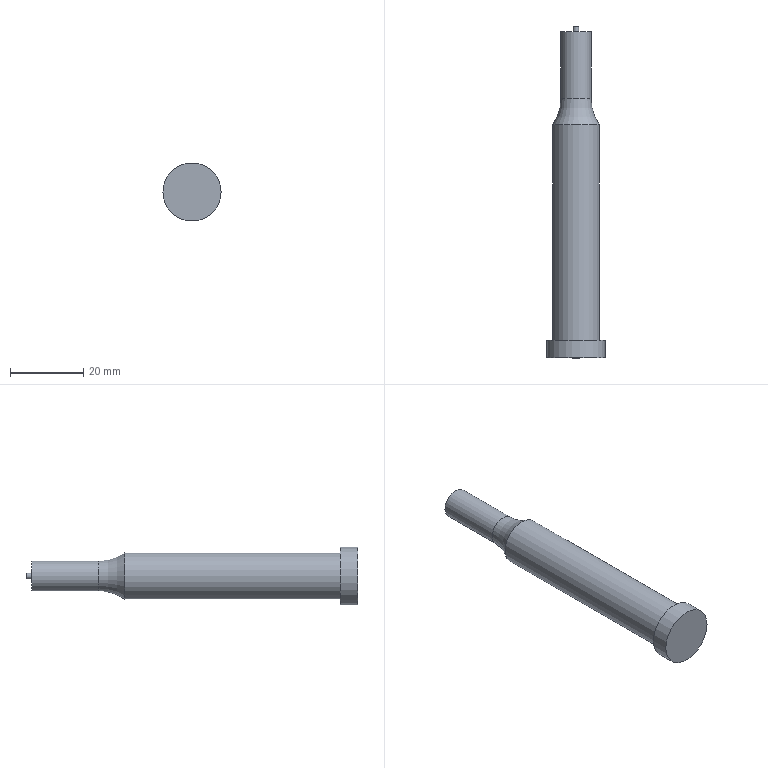Part | STEP file | 1_id1150_x_t | 1 solid | 9 faces | box 15.875 x 90.424 x 15.875 mm | volume 9884 mm3 | plane 4 | cylinder 4 | torus 1 | commonest cylinder face diameters 1.473 x1 8.199 x1 12.7 x1 15.875 x1
STEP:
#1=CARTESIAN_POINT('',(0.,0.,0.));
#2=DIRECTION('',(0.,0.,1.));
#3=DIRECTION('',(1.,0.,0.));
#4=AXIS2_PLACEMENT_3D('',#1,#2,#3);
#5=CARTESIAN_POINT('',(773.362,73.473,-70.67));
#6=VERTEX_POINT('',#5);
#7=CARTESIAN_POINT('',(757.487,73.473,-70.67));
#8=VERTEX_POINT('',#7);
#9=CARTESIAN_POINT('',(765.425,73.473,-70.67));
#10=DIRECTION('',(0.,-1.,0.));
#11=DIRECTION('',(1.,0.,0.));
#12=AXIS2_PLACEMENT_3D('',#9,#10,#11);
#13=CIRCLE('',#12,7.938);
#14=CARTESIAN_POINT('',(762.856,73.473,-70.67));
#15=DIRECTION('',(0.,-1.,0.));
#16=DIRECTION('',(1.,0.,0.));
#17=AXIS2_PLACEMENT_3D('',#14,#15,#16);
#18=PLANE('',#17);
#19=CARTESIAN_POINT('',(2.569,0.));
#20=DIRECTION('',(1.,0.));
#21=AXIS2_PLACEMENT_2D('',#19,#20);
#22=CIRCLE('',#21,7.938);
#23=(GEOMETRIC_REPRESENTATION_CONTEXT(2)PARAMETRIC_REPRESENTATION_CONTEXT()REPRESENTATION_CONTEXT('',''));
#24=DEFINITIONAL_REPRESENTATION('',(#22),#23);
#25=PCURVE('',#18,#24);
#26=CARTESIAN_POINT('',(765.425,75.861,-70.67));
#27=DIRECTION('',(0.,-1.,0.));
#28=DIRECTION('',(-1.,0.,0.));
#29=AXIS2_PLACEMENT_3D('',#26,#27,#28);
#30=CYLINDRICAL_SURFACE('',#29,7.938);
#31=CARTESIAN_POINT('',(3.142,2.388));
#32=DIRECTION('',(1.,0.));
#33=VECTOR('',#32,1.);
#34=LINE('',#31,#33);
#35=(GEOMETRIC_REPRESENTATION_CONTEXT(2)PARAMETRIC_REPRESENTATION_CONTEXT()REPRESENTATION_CONTEXT('',''));
#36=DEFINITIONAL_REPRESENTATION('',(#34),#35);
#37=PCURVE('',#30,#36);
#38=SURFACE_CURVE('',#13,(#25,#37),.PCURVE_S1.);
#39=EDGE_CURVE('',#6,#8,#38,.T.);
#40=ORIENTED_EDGE('',*,*,#39,.T.);
#41=CARTESIAN_POINT('',(765.425,73.473,-70.67));
#42=DIRECTION('',(0.,-1.,0.));
#43=DIRECTION('',(1.,0.,0.));
#44=AXIS2_PLACEMENT_3D('',#41,#42,#43);
#45=CIRCLE('',#44,7.938);
#46=CARTESIAN_POINT('',(2.569,0.));
#47=DIRECTION('',(1.,0.));
#48=AXIS2_PLACEMENT_2D('',#46,#47);
#49=CIRCLE('',#48,7.938);
#50=(GEOMETRIC_REPRESENTATION_CONTEXT(2)PARAMETRIC_REPRESENTATION_CONTEXT()REPRESENTATION_CONTEXT('',''));
#51=DEFINITIONAL_REPRESENTATION('',(#49),#50);
#52=PCURVE('',#18,#51);
#53=CARTESIAN_POINT('',(-3.142,2.388));
#54=DIRECTION('',(1.,0.));
#55=VECTOR('',#54,1.);
#56=LINE('',#53,#55);
#57=(GEOMETRIC_REPRESENTATION_CONTEXT(2)PARAMETRIC_REPRESENTATION_CONTEXT()REPRESENTATION_CONTEXT('',''));
#58=DEFINITIONAL_REPRESENTATION('',(#56),#57);
#59=PCURVE('',#30,#58);
#60=SURFACE_CURVE('',#45,(#52,#59),.PCURVE_S1.);
#61=EDGE_CURVE('',#8,#6,#60,.T.);
#62=ORIENTED_EDGE('',*,*,#61,.T.);
#63=EDGE_LOOP('',(#40,#62));
#64=FACE_BOUND('',#63,.T.);
#65=ADVANCED_FACE('',(#64),#18,.T.);
#66=CARTESIAN_POINT('',(757.487,78.248,-70.67));
#67=VERTEX_POINT('',#66);
#68=CARTESIAN_POINT('',(765.425,78.248,-70.67));
#69=DIRECTION('',(0.,1.,0.));
#70=DIRECTION('',(-1.,0.,0.));
#71=AXIS2_PLACEMENT_3D('',#68,#69,#70);
#72=CIRCLE('',#71,7.938);
#73=CARTESIAN_POINT('',(6.283,-2.388));
#74=DIRECTION('',(-1.,0.));
#75=VECTOR('',#74,1.);
#76=LINE('',#73,#75);
#77=(GEOMETRIC_REPRESENTATION_CONTEXT(2)PARAMETRIC_REPRESENTATION_CONTEXT()REPRESENTATION_CONTEXT('',''));
#78=DEFINITIONAL_REPRESENTATION('',(#76),#77);
#79=PCURVE('',#30,#78);
#80=CARTESIAN_POINT('',(727.581,78.248,-70.67));
#81=DIRECTION('',(0.,1.,0.));
#82=DIRECTION('',(1.,0.,0.));
#83=AXIS2_PLACEMENT_3D('',#80,#81,#82);
#84=PLANE('',#83);
#85=CARTESIAN_POINT('',(37.844,0.));
#86=DIRECTION('',(-1.,0.));
#87=AXIS2_PLACEMENT_2D('',#85,#86);
#88=CIRCLE('',#87,7.938);
#89=(GEOMETRIC_REPRESENTATION_CONTEXT(2)PARAMETRIC_REPRESENTATION_CONTEXT()REPRESENTATION_CONTEXT('',''));
#90=DEFINITIONAL_REPRESENTATION('',(#88),#89);
#91=PCURVE('',#84,#90);
#92=SURFACE_CURVE('',#72,(#79,#91),.PCURVE_S1.);
#93=EDGE_CURVE('',#67,#67,#92,.T.);
#94=ORIENTED_EDGE('',*,*,#93,.F.);
#95=CARTESIAN_POINT('',(757.487,78.248,-70.67));
#96=CARTESIAN_POINT('',(757.487,73.473,-70.67));
#97=B_SPLINE_CURVE_WITH_KNOTS('',1,(#95,#96),.UNSPECIFIED.,.F.,.F.,(2,2),(-2.388,2.388),.PIECEWISE_BEZIER_KNOTS.);
#98=CARTESIAN_POINT('',(6.283,0.));
#99=DIRECTION('',(0.,1.));
#100=VECTOR('',#99,1.);
#101=LINE('',#98,#100);
#102=(GEOMETRIC_REPRESENTATION_CONTEXT(2)PARAMETRIC_REPRESENTATION_CONTEXT()REPRESENTATION_CONTEXT('',''));
#103=DEFINITIONAL_REPRESENTATION('',(#101),#102);
#104=PCURVE('',#30,#103);
#105=CARTESIAN_POINT('',(0.,0.));
#106=DIRECTION('',(0.,1.));
#107=VECTOR('',#106,1.);
#108=LINE('',#105,#107);
#109=(GEOMETRIC_REPRESENTATION_CONTEXT(2)PARAMETRIC_REPRESENTATION_CONTEXT()REPRESENTATION_CONTEXT('',''));
#110=DEFINITIONAL_REPRESENTATION('',(#108),#109);
#111=PCURVE('',#30,#110);
#112=SEAM_CURVE('',#97,(#104,#111),.PCURVE_S1.);
#113=EDGE_CURVE('',#67,#8,#112,.T.);
#114=ORIENTED_EDGE('',*,*,#113,.T.);
#115=ORIENTED_EDGE('',*,*,#39,.F.);
#116=ORIENTED_EDGE('',*,*,#61,.F.);
#117=ORIENTED_EDGE('',*,*,#113,.F.);
#118=EDGE_LOOP('',(#94,#114,#115,#116,#117));
#119=FACE_BOUND('',#118,.T.);
#120=ADVANCED_FACE('',(#119),#30,.T.);
#121=ORIENTED_EDGE('',*,*,#93,.T.);
#122=EDGE_LOOP('',(#121));
#123=FACE_BOUND('',#122,.T.);
#124=CARTESIAN_POINT('',(771.775,78.248,-70.67));
#125=VERTEX_POINT('',#124);
#126=CARTESIAN_POINT('',(759.075,78.248,-70.67));
#127=VERTEX_POINT('',#126);
#128=CARTESIAN_POINT('',(765.425,78.248,-70.67));
#129=DIRECTION('',(0.,-1.,0.));
#130=DIRECTION('',(1.,0.,0.));
#131=AXIS2_PLACEMENT_3D('',#128,#129,#130);
#132=CIRCLE('',#131,6.35);
#133=CARTESIAN_POINT('',(44.194,0.));
#134=CARTESIAN_POINT('',(44.194,-10.999));
#135=CARTESIAN_POINT('',(34.669,-5.499));
#136=CARTESIAN_POINT('',(25.144,0.));
#137=CARTESIAN_POINT('',(34.669,5.499));
#138=CARTESIAN_POINT('',(44.194,10.999));
#139=CARTESIAN_POINT('',(44.194,0.));
#140=(BOUNDED_CURVE()B_SPLINE_CURVE(2,(#133,#134,#135,#136,#137,#138,#139),.UNSPECIFIED.,.T.,.F.)B_SPLINE_CURVE_WITH_KNOTS((1,2,2,2,2,1),(-2.094,0.,2.094,4.189,6.283,8.378),.UNSPECIFIED.)CURVE()GEOMETRIC_REPRESENTATION_ITEM()RATIONAL_B_SPLINE_CURVE((1.,0.5,1.,0.5,1.,0.5,1.))REPRESENTATION_ITEM(''));
#141=(GEOMETRIC_REPRESENTATION_CONTEXT(2)PARAMETRIC_REPRESENTATION_CONTEXT()REPRESENTATION_CONTEXT('',''));
#142=DEFINITIONAL_REPRESENTATION('',(#140),#141);
#143=PCURVE('',#84,#142);
#144=CARTESIAN_POINT('',(765.425,107.611,-70.67));
#145=DIRECTION('',(0.,-1.,0.));
#146=DIRECTION('',(-1.,0.,0.));
#147=AXIS2_PLACEMENT_3D('',#144,#145,#146);
#148=CYLINDRICAL_SURFACE('',#147,6.35);
#149=CARTESIAN_POINT('',(3.142,29.362));
#150=DIRECTION('',(1.,0.));
#151=VECTOR('',#150,1.);
#152=LINE('',#149,#151);
#153=(GEOMETRIC_REPRESENTATION_CONTEXT(2)PARAMETRIC_REPRESENTATION_CONTEXT()REPRESENTATION_CONTEXT('',''));
#154=DEFINITIONAL_REPRESENTATION('',(#152),#153);
#155=PCURVE('',#148,#154);
#156=SURFACE_CURVE('',#132,(#143,#155),.PCURVE_S1.);
#157=EDGE_CURVE('',#125,#127,#156,.T.);
#158=ORIENTED_EDGE('',*,*,#157,.T.);
#159=CARTESIAN_POINT('',(765.425,78.248,-70.67));
#160=DIRECTION('',(0.,-1.,0.));
#161=DIRECTION('',(1.,0.,0.));
#162=AXIS2_PLACEMENT_3D('',#159,#160,#161);
#163=CIRCLE('',#162,6.35);
#164=CARTESIAN_POINT('',(44.194,0.));
#165=CARTESIAN_POINT('',(44.194,-10.999));
#166=CARTESIAN_POINT('',(34.669,-5.499));
#167=CARTESIAN_POINT('',(25.144,0.));
#168=CARTESIAN_POINT('',(34.669,5.499));
#169=CARTESIAN_POINT('',(44.194,10.999));
#170=CARTESIAN_POINT('',(44.194,0.));
#171=(BOUNDED_CURVE()B_SPLINE_CURVE(2,(#164,#165,#166,#167,#168,#169,#170),.UNSPECIFIED.,.T.,.F.)B_SPLINE_CURVE_WITH_KNOTS((1,2,2,2,2,1),(-2.094,0.,2.094,4.189,6.283,8.378),.UNSPECIFIED.)CURVE()GEOMETRIC_REPRESENTATION_ITEM()RATIONAL_B_SPLINE_CURVE((1.,0.5,1.,0.5,1.,0.5,1.))REPRESENTATION_ITEM(''));
#172=(GEOMETRIC_REPRESENTATION_CONTEXT(2)PARAMETRIC_REPRESENTATION_CONTEXT()REPRESENTATION_CONTEXT('',''));
#173=DEFINITIONAL_REPRESENTATION('',(#171),#172);
#174=PCURVE('',#84,#173);
#175=CARTESIAN_POINT('',(-3.142,29.362));
#176=DIRECTION('',(1.,0.));
#177=VECTOR('',#176,1.);
#178=LINE('',#175,#177);
#179=(GEOMETRIC_REPRESENTATION_CONTEXT(2)PARAMETRIC_REPRESENTATION_CONTEXT()REPRESENTATION_CONTEXT('',''));
#180=DEFINITIONAL_REPRESENTATION('',(#178),#179);
#181=PCURVE('',#148,#180);
#182=SURFACE_CURVE('',#163,(#174,#181),.PCURVE_S1.);
#183=EDGE_CURVE('',#127,#125,#182,.T.);
#184=ORIENTED_EDGE('',*,*,#183,.T.);
#185=EDGE_LOOP('',(#158,#184));
#186=FACE_BOUND('',#185,.T.);
#187=ADVANCED_FACE('',(#123,#186),#84,.T.);
#188=ORIENTED_EDGE('',*,*,#183,.F.);
#189=CARTESIAN_POINT('',(759.075,136.973,-70.67));
#190=VERTEX_POINT('',#189);
#191=CARTESIAN_POINT('',(759.075,136.973,-70.67));
#192=CARTESIAN_POINT('',(759.075,78.248,-70.67));
#193=B_SPLINE_CURVE_WITH_KNOTS('',1,(#191,#192),.UNSPECIFIED.,.F.,.F.,(2,2),(-29.362,29.362),.PIECEWISE_BEZIER_KNOTS.);
#194=CARTESIAN_POINT('',(0.,0.));
#195=DIRECTION('',(0.,1.));
#196=VECTOR('',#195,1.);
#197=LINE('',#194,#196);
#198=(GEOMETRIC_REPRESENTATION_CONTEXT(2)PARAMETRIC_REPRESENTATION_CONTEXT()REPRESENTATION_CONTEXT('',''));
#199=DEFINITIONAL_REPRESENTATION('',(#197),#198);
#200=PCURVE('',#148,#199);
#201=CARTESIAN_POINT('',(6.283,0.));
#202=DIRECTION('',(0.,1.));
#203=VECTOR('',#202,1.);
#204=LINE('',#201,#203);
#205=(GEOMETRIC_REPRESENTATION_CONTEXT(2)PARAMETRIC_REPRESENTATION_CONTEXT()REPRESENTATION_CONTEXT('',''));
#206=DEFINITIONAL_REPRESENTATION('',(#204),#205);
#207=PCURVE('',#148,#206);
#208=SEAM_CURVE('',#193,(#200,#207),.PCURVE_S1.);
#209=EDGE_CURVE('',#190,#127,#208,.T.);
#210=ORIENTED_EDGE('',*,*,#209,.F.);
#211=CARTESIAN_POINT('',(771.775,136.973,-70.67));
#212=VERTEX_POINT('',#211);
#213=CARTESIAN_POINT('',(765.425,136.973,-70.67));
#214=DIRECTION('',(0.,1.,0.));
#215=DIRECTION('',(-1.,0.,0.));
#216=AXIS2_PLACEMENT_3D('',#213,#214,#215);
#217=CIRCLE('',#216,6.35);
#218=CARTESIAN_POINT('',(6.283,-29.362));
#219=DIRECTION('',(-1.,0.));
#220=VECTOR('',#219,1.);
#221=LINE('',#218,#220);
#222=(GEOMETRIC_REPRESENTATION_CONTEXT(2)PARAMETRIC_REPRESENTATION_CONTEXT()REPRESENTATION_CONTEXT('',''));
#223=DEFINITIONAL_REPRESENTATION('',(#221),#222);
#224=PCURVE('',#148,#223);
#225=CARTESIAN_POINT('',(765.425,144.191,-70.67));
#226=DIRECTION('',(0.,-1.,0.));
#227=DIRECTION('',(1.,0.,0.));
#228=AXIS2_PLACEMENT_3D('',#225,#226,#227);
#229=TOROIDAL_SURFACE('',#228,16.8,12.7);
#230=CARTESIAN_POINT('',(9.425,8.82));
#231=DIRECTION('',(-1.,0.));
#232=VECTOR('',#231,1.);
#233=LINE('',#230,#232);
#234=(GEOMETRIC_REPRESENTATION_CONTEXT(2)PARAMETRIC_REPRESENTATION_CONTEXT()REPRESENTATION_CONTEXT('',''));
#235=DEFINITIONAL_REPRESENTATION('',(#233),#234);
#236=PCURVE('',#229,#235);
#237=SURFACE_CURVE('',#217,(#224,#236),.PCURVE_S1.);
#238=EDGE_CURVE('',#212,#190,#237,.T.);
#239=ORIENTED_EDGE('',*,*,#238,.F.);
#240=CARTESIAN_POINT('',(765.425,136.973,-70.67));
#241=DIRECTION('',(0.,1.,0.));
#242=DIRECTION('',(-1.,0.,0.));
#243=AXIS2_PLACEMENT_3D('',#240,#241,#242);
#244=CIRCLE('',#243,6.35);
#245=CARTESIAN_POINT('',(6.283,-29.362));
#246=DIRECTION('',(-1.,0.));
#247=VECTOR('',#246,1.);
#248=LINE('',#245,#247);
#249=(GEOMETRIC_REPRESENTATION_CONTEXT(2)PARAMETRIC_REPRESENTATION_CONTEXT()REPRESENTATION_CONTEXT('',''));
#250=DEFINITIONAL_REPRESENTATION('',(#248),#249);
#251=PCURVE('',#148,#250);
#252=CARTESIAN_POINT('',(3.142,8.82));
#253=DIRECTION('',(-1.,0.));
#254=VECTOR('',#253,1.);
#255=LINE('',#252,#254);
#256=(GEOMETRIC_REPRESENTATION_CONTEXT(2)PARAMETRIC_REPRESENTATION_CONTEXT()REPRESENTATION_CONTEXT('',''));
#257=DEFINITIONAL_REPRESENTATION('',(#255),#256);
#258=PCURVE('',#229,#257);
#259=SURFACE_CURVE('',#244,(#251,#258),.PCURVE_S1.);
#260=EDGE_CURVE('',#190,#212,#259,.T.);
#261=ORIENTED_EDGE('',*,*,#260,.F.);
#262=ORIENTED_EDGE('',*,*,#209,.T.);
#263=ORIENTED_EDGE('',*,*,#157,.F.);
#264=EDGE_LOOP('',(#188,#210,#239,#261,#262,#263));
#265=FACE_BOUND('',#264,.T.);
#266=ADVANCED_FACE('',(#265),#148,.T.);
#267=CARTESIAN_POINT('',(769.525,144.191,-70.67));
#268=VERTEX_POINT('',#267);
#269=CARTESIAN_POINT('',(761.325,144.191,-70.67));
#270=VERTEX_POINT('',#269);
#271=CARTESIAN_POINT('',(765.425,144.191,-70.67));
#272=DIRECTION('',(0.,-1.,0.));
#273=DIRECTION('',(1.,0.,0.));
#274=AXIS2_PLACEMENT_3D('',#271,#272,#273);
#275=CIRCLE('',#274,4.1);
#276=CARTESIAN_POINT('',(0.,9.425));
#277=DIRECTION('',(1.,0.));
#278=VECTOR('',#277,1.);
#279=LINE('',#276,#278);
#280=(GEOMETRIC_REPRESENTATION_CONTEXT(2)PARAMETRIC_REPRESENTATION_CONTEXT()REPRESENTATION_CONTEXT('',''));
#281=DEFINITIONAL_REPRESENTATION('',(#279),#280);
#282=PCURVE('',#229,#281);
#283=CARTESIAN_POINT('',(765.425,153.282,-70.67));
#284=DIRECTION('',(0.,-1.,0.));
#285=DIRECTION('',(-1.,0.,0.));
#286=AXIS2_PLACEMENT_3D('',#283,#284,#285);
#287=CYLINDRICAL_SURFACE('',#286,4.1);
#288=CARTESIAN_POINT('',(3.142,9.091));
#289=DIRECTION('',(1.,0.));
#290=VECTOR('',#289,1.);
#291=LINE('',#288,#290);
#292=(GEOMETRIC_REPRESENTATION_CONTEXT(2)PARAMETRIC_REPRESENTATION_CONTEXT()REPRESENTATION_CONTEXT('',''));
#293=DEFINITIONAL_REPRESENTATION('',(#291),#292);
#294=PCURVE('',#287,#293);
#295=SURFACE_CURVE('',#275,(#282,#294),.PCURVE_S1.);
#296=EDGE_CURVE('',#268,#270,#295,.T.);
#297=ORIENTED_EDGE('',*,*,#296,.F.);
#298=CARTESIAN_POINT('',(771.775,136.973,-70.67));
#299=CARTESIAN_POINT('',(771.046,138.029,-70.67));
#300=CARTESIAN_POINT('',(770.447,139.169,-70.67));
#301=CARTESIAN_POINT('',(769.989,140.376,-70.67));
#302=CARTESIAN_POINT('',(769.68,141.629,-70.67));
#303=CARTESIAN_POINT('',(769.525,142.907,-70.67));
#304=CARTESIAN_POINT('',(769.525,144.191,-70.67));
#305=(BOUNDED_CURVE()B_SPLINE_CURVE(6,(#298,#299,#300,#301,#302,#303,#304),.UNSPECIFIED.,.F.,.F.)B_SPLINE_CURVE_WITH_KNOTS((7,7),(2.537,3.142),.PIECEWISE_BEZIER_KNOTS.)CURVE()GEOMETRIC_REPRESENTATION_ITEM()RATIONAL_B_SPLINE_CURVE((1.005,1.002,0.9997,0.9991,0.9997,1.002,1.005))REPRESENTATION_ITEM(''));
#306=CARTESIAN_POINT('',(0.,6.283));
#307=DIRECTION('',(0.,1.));
#308=VECTOR('',#307,1.);
#309=LINE('',#306,#308);
#310=(GEOMETRIC_REPRESENTATION_CONTEXT(2)PARAMETRIC_REPRESENTATION_CONTEXT()REPRESENTATION_CONTEXT('',''));
#311=DEFINITIONAL_REPRESENTATION('',(#309),#310);
#312=PCURVE('',#229,#311);
#313=CARTESIAN_POINT('',(6.283,6.283));
#314=DIRECTION('',(0.,1.));
#315=VECTOR('',#314,1.);
#316=LINE('',#313,#315);
#317=(GEOMETRIC_REPRESENTATION_CONTEXT(2)PARAMETRIC_REPRESENTATION_CONTEXT()REPRESENTATION_CONTEXT('',''));
#318=DEFINITIONAL_REPRESENTATION('',(#316),#317);
#319=PCURVE('',#229,#318);
#320=SEAM_CURVE('',#305,(#312,#319),.PCURVE_S1.);
#321=EDGE_CURVE('',#212,#268,#320,.T.);
#322=ORIENTED_EDGE('',*,*,#321,.F.);
#323=ORIENTED_EDGE('',*,*,#260,.F.);
#324=ORIENTED_EDGE('',*,*,#238,.F.);
#325=ORIENTED_EDGE('',*,*,#321,.T.);
#326=CARTESIAN_POINT('',(765.425,144.191,-70.67));
#327=DIRECTION('',(0.,-1.,0.));
#328=DIRECTION('',(1.,0.,0.));
#329=AXIS2_PLACEMENT_3D('',#326,#327,#328);
#330=CIRCLE('',#329,4.1);
#331=CARTESIAN_POINT('',(0.,9.425));
#332=DIRECTION('',(1.,0.));
#333=VECTOR('',#332,1.);
#334=LINE('',#331,#333);
#335=(GEOMETRIC_REPRESENTATION_CONTEXT(2)PARAMETRIC_REPRESENTATION_CONTEXT()REPRESENTATION_CONTEXT('',''));
#336=DEFINITIONAL_REPRESENTATION('',(#334),#335);
#337=PCURVE('',#229,#336);
#338=CARTESIAN_POINT('',(-3.142,9.091));
#339=DIRECTION('',(1.,0.));
#340=VECTOR('',#339,1.);
#341=LINE('',#338,#340);
#342=(GEOMETRIC_REPRESENTATION_CONTEXT(2)PARAMETRIC_REPRESENTATION_CONTEXT()REPRESENTATION_CONTEXT('',''));
#343=DEFINITIONAL_REPRESENTATION('',(#341),#342);
#344=PCURVE('',#287,#343);
#345=SURFACE_CURVE('',#330,(#337,#344),.PCURVE_S1.);
#346=EDGE_CURVE('',#270,#268,#345,.T.);
#347=ORIENTED_EDGE('',*,*,#346,.F.);
#348=EDGE_LOOP('',(#297,#322,#323,#324,#325,#347));
#349=FACE_BOUND('',#348,.F.);
#350=ADVANCED_FACE('',(#349),#229,.F.);
#351=CARTESIAN_POINT('',(761.325,162.373,-70.67));
#352=VERTEX_POINT('',#351);
#353=CARTESIAN_POINT('',(765.425,162.373,-70.67));
#354=DIRECTION('',(0.,1.,0.));
#355=DIRECTION('',(-1.,0.,0.));
#356=AXIS2_PLACEMENT_3D('',#353,#354,#355);
#357=CIRCLE('',#356,4.1);
#358=CARTESIAN_POINT('',(6.283,-9.091));
#359=DIRECTION('',(-1.,0.));
#360=VECTOR('',#359,1.);
#361=LINE('',#358,#360);
#362=(GEOMETRIC_REPRESENTATION_CONTEXT(2)PARAMETRIC_REPRESENTATION_CONTEXT()REPRESENTATION_CONTEXT('',''));
#363=DEFINITIONAL_REPRESENTATION('',(#361),#362);
#364=PCURVE('',#287,#363);
#365=CARTESIAN_POINT('',(763.375,162.373,-70.67));
#366=DIRECTION('',(0.,1.,0.));
#367=DIRECTION('',(1.,0.,0.));
#368=AXIS2_PLACEMENT_3D('',#365,#366,#367);
#369=PLANE('',#368);
#370=CARTESIAN_POINT('',(2.05,0.));
#371=DIRECTION('',(-1.,0.));
#372=AXIS2_PLACEMENT_2D('',#370,#371);
#373=CIRCLE('',#372,4.1);
#374=(GEOMETRIC_REPRESENTATION_CONTEXT(2)PARAMETRIC_REPRESENTATION_CONTEXT()REPRESENTATION_CONTEXT('',''));
#375=DEFINITIONAL_REPRESENTATION('',(#373),#374);
#376=PCURVE('',#369,#375);
#377=SURFACE_CURVE('',#357,(#364,#376),.PCURVE_S1.);
#378=EDGE_CURVE('',#352,#352,#377,.T.);
#379=ORIENTED_EDGE('',*,*,#378,.F.);
#380=CARTESIAN_POINT('',(761.325,162.373,-70.67));
#381=CARTESIAN_POINT('',(761.325,144.191,-70.67));
#382=B_SPLINE_CURVE_WITH_KNOTS('',1,(#380,#381),.UNSPECIFIED.,.F.,.F.,(2,2),(-9.091,9.091),.PIECEWISE_BEZIER_KNOTS.);
#383=CARTESIAN_POINT('',(6.283,0.));
#384=DIRECTION('',(0.,1.));
#385=VECTOR('',#384,1.);
#386=LINE('',#383,#385);
#387=(GEOMETRIC_REPRESENTATION_CONTEXT(2)PARAMETRIC_REPRESENTATION_CONTEXT()REPRESENTATION_CONTEXT('',''));
#388=DEFINITIONAL_REPRESENTATION('',(#386),#387);
#389=PCURVE('',#287,#388);
#390=CARTESIAN_POINT('',(0.,0.));
#391=DIRECTION('',(0.,1.));
#392=VECTOR('',#391,1.);
#393=LINE('',#390,#392);
#394=(GEOMETRIC_REPRESENTATION_CONTEXT(2)PARAMETRIC_REPRESENTATION_CONTEXT()REPRESENTATION_CONTEXT('',''));
#395=DEFINITIONAL_REPRESENTATION('',(#393),#394);
#396=PCURVE('',#287,#395);
#397=SEAM_CURVE('',#382,(#389,#396),.PCURVE_S1.);
#398=EDGE_CURVE('',#352,#270,#397,.T.);
#399=ORIENTED_EDGE('',*,*,#398,.T.);
#400=ORIENTED_EDGE('',*,*,#296,.F.);
#401=ORIENTED_EDGE('',*,*,#346,.F.);
#402=ORIENTED_EDGE('',*,*,#398,.F.);
#403=EDGE_LOOP('',(#379,#399,#400,#401,#402));
#404=FACE_BOUND('',#403,.T.);
#405=ADVANCED_FACE('',(#404),#287,.T.);
#406=ORIENTED_EDGE('',*,*,#378,.T.);
#407=EDGE_LOOP('',(#406));
#408=FACE_BOUND('',#407,.T.);
#409=CARTESIAN_POINT('',(766.162,162.373,-70.67));
#410=VERTEX_POINT('',#409);
#411=CARTESIAN_POINT('',(765.425,162.373,-70.67));
#412=DIRECTION('',(0.,-1.,0.));
#413=DIRECTION('',(1.,0.,0.));
#414=AXIS2_PLACEMENT_3D('',#411,#412,#413);
#415=CIRCLE('',#414,0.7366);
#416=CARTESIAN_POINT('',(2.786,0.));
#417=CARTESIAN_POINT('',(2.786,-1.276));
#418=CARTESIAN_POINT('',(1.681,-0.6379));
#419=CARTESIAN_POINT('',(0.5766,0.));
#420=CARTESIAN_POINT('',(1.681,0.6379));
#421=CARTESIAN_POINT('',(2.786,1.276));
#422=CARTESIAN_POINT('',(2.786,0.));
#423=(BOUNDED_CURVE()B_SPLINE_CURVE(2,(#416,#417,#418,#419,#420,#421,#422),.UNSPECIFIED.,.T.,.F.)B_SPLINE_CURVE_WITH_KNOTS((1,2,2,2,2,1),(-2.094,0.,2.094,4.189,6.283,8.378),.UNSPECIFIED.)CURVE()GEOMETRIC_REPRESENTATION_ITEM()RATIONAL_B_SPLINE_CURVE((1.,0.5,1.,0.5,1.,0.5,1.))REPRESENTATION_ITEM(''));
#424=(GEOMETRIC_REPRESENTATION_CONTEXT(2)PARAMETRIC_REPRESENTATION_CONTEXT()REPRESENTATION_CONTEXT('',''));
#425=DEFINITIONAL_REPRESENTATION('',(#423),#424);
#426=PCURVE('',#369,#425);
#427=CARTESIAN_POINT('',(765.425,160.849,-70.67));
#428=DIRECTION('',(0.,1.,0.));
#429=DIRECTION('',(1.,0.,0.));
#430=AXIS2_PLACEMENT_3D('',#427,#428,#429);
#431=CYLINDRICAL_SURFACE('',#430,0.7366);
#432=CARTESIAN_POINT('',(6.283,1.524));
#433=DIRECTION('',(-1.,0.));
#434=VECTOR('',#433,1.);
#435=LINE('',#432,#434);
#436=(GEOMETRIC_REPRESENTATION_CONTEXT(2)PARAMETRIC_REPRESENTATION_CONTEXT()REPRESENTATION_CONTEXT('',''));
#437=DEFINITIONAL_REPRESENTATION('',(#435),#436);
#438=PCURVE('',#431,#437);
#439=SURFACE_CURVE('',#415,(#426,#438),.PCURVE_S1.);
#440=EDGE_CURVE('',#410,#410,#439,.T.);
#441=ORIENTED_EDGE('',*,*,#440,.T.);
#442=EDGE_LOOP('',(#441));
#443=FACE_BOUND('',#442,.T.);
#444=ADVANCED_FACE('',(#408,#443),#369,.T.);
#445=ORIENTED_EDGE('',*,*,#440,.F.);
#446=CARTESIAN_POINT('',(766.162,163.897,-70.67));
#447=VERTEX_POINT('',#446);
#448=CARTESIAN_POINT('',(766.162,162.373,-70.67));
#449=CARTESIAN_POINT('',(766.162,163.897,-70.67));
#450=B_SPLINE_CURVE_WITH_KNOTS('',1,(#448,#449),.UNSPECIFIED.,.F.,.F.,(2,2),(1.524,3.048),.PIECEWISE_BEZIER_KNOTS.);
#451=CARTESIAN_POINT('',(6.283,0.));
#452=DIRECTION('',(0.,1.));
#453=VECTOR('',#452,1.);
#454=LINE('',#451,#453);
#455=(GEOMETRIC_REPRESENTATION_CONTEXT(2)PARAMETRIC_REPRESENTATION_CONTEXT()REPRESENTATION_CONTEXT('',''));
#456=DEFINITIONAL_REPRESENTATION('',(#454),#455);
#457=PCURVE('',#431,#456);
#458=CARTESIAN_POINT('',(0.,0.));
#459=DIRECTION('',(0.,1.));
#460=VECTOR('',#459,1.);
#461=LINE('',#458,#460);
#462=(GEOMETRIC_REPRESENTATION_CONTEXT(2)PARAMETRIC_REPRESENTATION_CONTEXT()REPRESENTATION_CONTEXT('',''));
#463=DEFINITIONAL_REPRESENTATION('',(#461),#462);
#464=PCURVE('',#431,#463);
#465=SEAM_CURVE('',#450,(#457,#464),.PCURVE_S1.);
#466=EDGE_CURVE('',#410,#447,#465,.T.);
#467=ORIENTED_EDGE('',*,*,#466,.T.);
#468=CARTESIAN_POINT('',(764.688,163.897,-70.67));
#469=VERTEX_POINT('',#468);
#470=CARTESIAN_POINT('',(765.425,163.897,-70.67));
#471=DIRECTION('',(0.,1.,0.));
#472=DIRECTION('',(-1.,0.,0.));
#473=AXIS2_PLACEMENT_3D('',#470,#471,#472);
#474=CIRCLE('',#473,0.7366);
#475=CARTESIAN_POINT('',(3.142,3.048));
#476=DIRECTION('',(1.,0.));
#477=VECTOR('',#476,1.);
#478=LINE('',#475,#477);
#479=(GEOMETRIC_REPRESENTATION_CONTEXT(2)PARAMETRIC_REPRESENTATION_CONTEXT()REPRESENTATION_CONTEXT('',''));
#480=DEFINITIONAL_REPRESENTATION('',(#478),#479);
#481=PCURVE('',#431,#480);
#482=CARTESIAN_POINT('',(765.425,163.897,-70.67));
#483=DIRECTION('',(0.,-1.,0.));
#484=DIRECTION('',(1.,0.,0.));
#485=AXIS2_PLACEMENT_3D('',#482,#483,#484);
#486=PLANE('',#485);
#487=CARTESIAN_POINT('',(-0.7366,0.));
#488=CARTESIAN_POINT('',(-0.7366,1.276));
#489=CARTESIAN_POINT('',(0.3683,0.6379));
#490=CARTESIAN_POINT('',(1.473,0.));
#491=CARTESIAN_POINT('',(0.3683,-0.6379));
#492=CARTESIAN_POINT('',(-0.7366,-1.276));
#493=CARTESIAN_POINT('',(-0.7366,0.));
#494=(BOUNDED_CURVE()B_SPLINE_CURVE(2,(#487,#488,#489,#490,#491,#492,#493),.UNSPECIFIED.,.T.,.F.)B_SPLINE_CURVE_WITH_KNOTS((1,2,2,2,2,1),(-2.094,0.,2.094,4.189,6.283,8.378),.UNSPECIFIED.)CURVE()GEOMETRIC_REPRESENTATION_ITEM()RATIONAL_B_SPLINE_CURVE((1.,0.5,1.,0.5,1.,0.5,1.))REPRESENTATION_ITEM(''));
#495=(GEOMETRIC_REPRESENTATION_CONTEXT(2)PARAMETRIC_REPRESENTATION_CONTEXT()REPRESENTATION_CONTEXT('',''));
#496=DEFINITIONAL_REPRESENTATION('',(#494),#495);
#497=PCURVE('',#486,#496);
#498=SURFACE_CURVE('',#474,(#481,#497),.PCURVE_S1.);
#499=EDGE_CURVE('',#469,#447,#498,.T.);
#500=ORIENTED_EDGE('',*,*,#499,.F.);
#501=CARTESIAN_POINT('',(765.425,163.897,-70.67));
#502=DIRECTION('',(0.,1.,0.));
#503=DIRECTION('',(-1.,0.,0.));
#504=AXIS2_PLACEMENT_3D('',#501,#502,#503);
#505=CIRCLE('',#504,0.7366);
#506=CARTESIAN_POINT('',(-3.142,3.048));
#507=DIRECTION('',(1.,0.));
#508=VECTOR('',#507,1.);
#509=LINE('',#506,#508);
#510=(GEOMETRIC_REPRESENTATION_CONTEXT(2)PARAMETRIC_REPRESENTATION_CONTEXT()REPRESENTATION_CONTEXT('',''));
#511=DEFINITIONAL_REPRESENTATION('',(#509),#510);
#512=PCURVE('',#431,#511);
#513=CARTESIAN_POINT('',(-0.7366,0.));
#514=CARTESIAN_POINT('',(-0.7366,1.276));
#515=CARTESIAN_POINT('',(0.3683,0.6379));
#516=CARTESIAN_POINT('',(1.473,0.));
#517=CARTESIAN_POINT('',(0.3683,-0.6379));
#518=CARTESIAN_POINT('',(-0.7366,-1.276));
#519=CARTESIAN_POINT('',(-0.7366,0.));
#520=(BOUNDED_CURVE()B_SPLINE_CURVE(2,(#513,#514,#515,#516,#517,#518,#519),.UNSPECIFIED.,.T.,.F.)B_SPLINE_CURVE_WITH_KNOTS((1,2,2,2,2,1),(-2.094,0.,2.094,4.189,6.283,8.378),.UNSPECIFIED.)CURVE()GEOMETRIC_REPRESENTATION_ITEM()RATIONAL_B_SPLINE_CURVE((1.,0.5,1.,0.5,1.,0.5,1.))REPRESENTATION_ITEM(''));
#521=(GEOMETRIC_REPRESENTATION_CONTEXT(2)PARAMETRIC_REPRESENTATION_CONTEXT()REPRESENTATION_CONTEXT('',''));
#522=DEFINITIONAL_REPRESENTATION('',(#520),#521);
#523=PCURVE('',#486,#522);
#524=SURFACE_CURVE('',#505,(#512,#523),.PCURVE_S1.);
#525=EDGE_CURVE('',#447,#469,#524,.T.);
#526=ORIENTED_EDGE('',*,*,#525,.F.);
#527=ORIENTED_EDGE('',*,*,#466,.F.);
#528=EDGE_LOOP('',(#445,#467,#500,#526,#527));
#529=FACE_BOUND('',#528,.T.);
#530=ADVANCED_FACE('',(#529),#431,.T.);
#531=ORIENTED_EDGE('',*,*,#499,.T.);
#532=ORIENTED_EDGE('',*,*,#525,.T.);
#533=EDGE_LOOP('',(#531,#532));
#534=FACE_BOUND('',#533,.T.);
#535=ADVANCED_FACE('',(#534),#486,.F.);
#536=CLOSED_SHELL('',(#65,#120,#187,#266,#350,#405,#444,#530,#535));
#537=MANIFOLD_SOLID_BREP('',#536);
#538=(LENGTH_UNIT()NAMED_UNIT(*)SI_UNIT(.MILLI.,.METRE.));
#539=UNCERTAINTY_MEASURE_WITH_UNIT(LENGTH_MEASURE(0.000005),#538,'','');
#540=(NAMED_UNIT(*)PLANE_ANGLE_UNIT()SI_UNIT($,.RADIAN.));
#541=(NAMED_UNIT(*)SI_UNIT($,.STERADIAN.)SOLID_ANGLE_UNIT());
#542=(GEOMETRIC_REPRESENTATION_CONTEXT(3)GLOBAL_UNCERTAINTY_ASSIGNED_CONTEXT((#539))GLOBAL_UNIT_ASSIGNED_CONTEXT((#538,#540,#541))REPRESENTATION_CONTEXT('',''));
#543=ADVANCED_BREP_SHAPE_REPRESENTATION('',(#4,#537),#542);